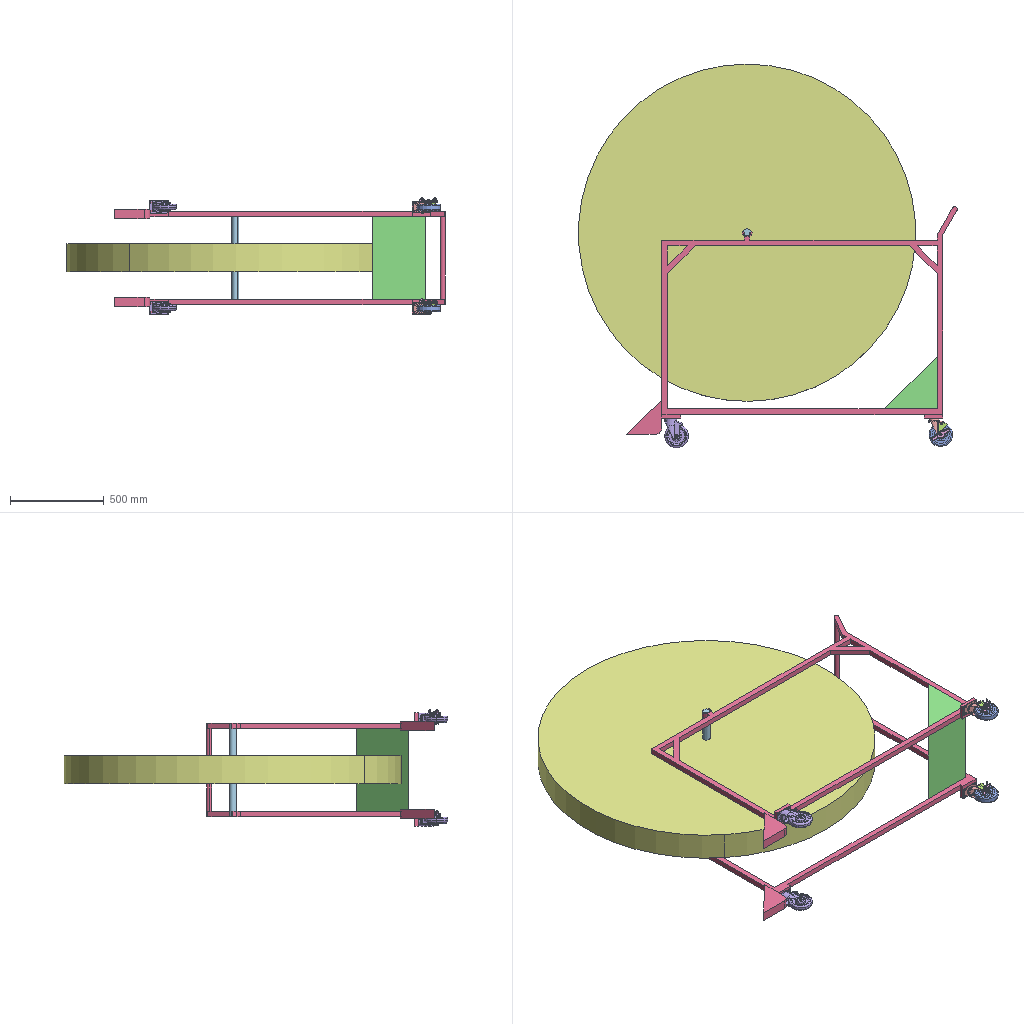Assembly | SolidWorks | 13 different items | 20 placed | box 2020 x 2048 x 623 mm
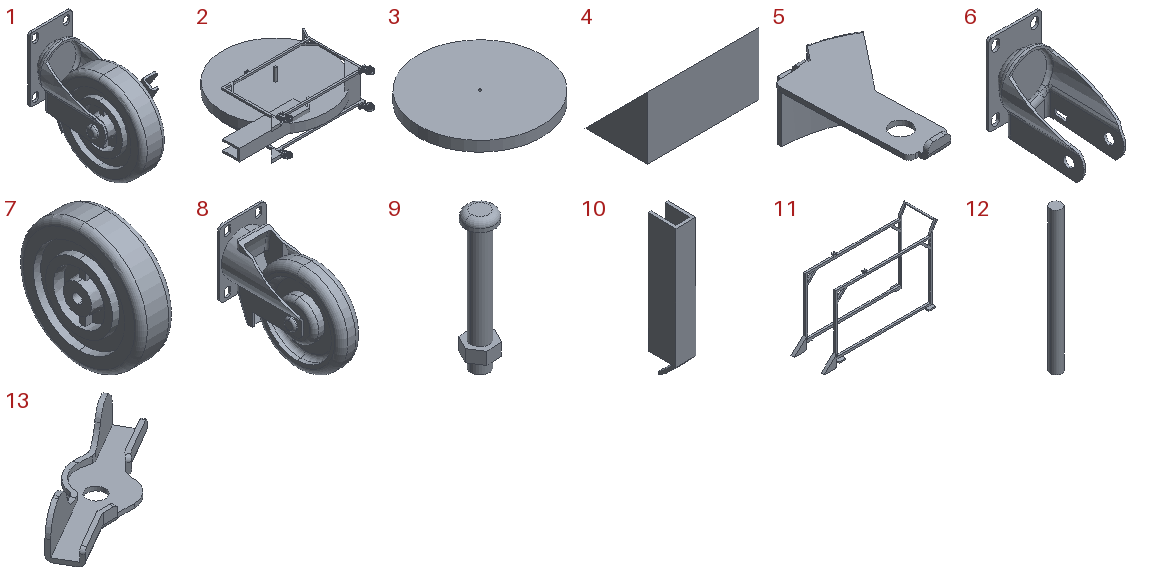Parts list (item | name | quantity | parent item | size | volume | features):
1 | (subassembly) | x2 | - | 82.741 x 151.003 x 143.701 mm | 434028 mm3 | features AEMSimFeature 1, CompositeCurve 1
2 | (subassembly) | x1 | - | 2265 x 1855 x 622.797 mm | 442404059 mm3 | -
3 | - | x1 | - | 1800 x 1800 x 150 mm | 381515012 mm3 | features Extrusion 1, ICE 1
4 | - | x1 | - | 500 x 280 x 280 mm | 19600000 mm3 | features ICE 4, Extrusion 1
5 | - | x2 | in 1 | 48.773 x 87.122 x 45.946 mm | 8989 mm3 | features Fillet 2, ICE 2, SM3dBend 2, FlatPattern 1, SMBaseFlange 1, SheetMetal 1
6 | - | x2 | in 1 | 62.612 x 104.648 x 97.984 mm | 58421 mm3 | features ICE 8, Fillet 5, Extrusion 1, RevCut 1, Revolution 1, Shell 1
7 | - | x2 | in 1 | 37.592 x 125.73 x 125.73 mm | 351247 mm3 | features Cut 2, Draft 2, ICE 2, BossThin 1, Extrusion 1, Fillet 1, MirrorPattern 1
8 | - | x2 | - | 66.675 x 158.75 x 142.081 mm | 379574 mm3 | features ICE 12, Fillet 8, MirrorPattern 5, Extrusion 1, RevCut 1
9 | - | x2 | in 1 | 16.107 x 15.24 x 71.12 mm | 6159 mm3 | features ICE 2, Extrusion 1, Fillet 1
10 | - | x1 | - | 200 x 280 x 1354 mm | 26886001 mm3 | features ICE 3, Extrusion 1
11 | - | x1 | - | 1767 x 605.941 x 1214 mm | 12147544 mm3 | features ICE 12, MirrorPattern 4, Extrusion 1, Fillet 1
12 | - | x1 | - | 40 x 40 x 500 mm | 628319 mm3 | features Extrusion 1
13 | - | x2 | in 1 | 96.878 x 66.198 x 24.765 mm | 9212 mm3 | features Fillet 4, ICE 4, Cut 1, FlatPattern 1, SMBaseFlange 1, SheetMetal 1
Mates (type | each side: item.copy, entity, surface, feature):
In the top assembly
Coincident | 4.1 face plane Boss-Extrude1 | 11.1 face plane Boss-Extrude1 | 2 times
Coincident | 11.1 face plane Boss-Extrude1 | 12.1 face plane Boss-Extrude1
Concentric | 12.1 face cylinder Boss-Extrude1 | 3.1 face cylinder Cut-Extrude1
Coincident | 4.1 face plane Boss-Extrude1 | 11.1 face plane Boss-Extrude2
DistanceDim | 11.1 face plane Boss-Extrude1 | 3.1 face plane Boss-Extrude1
Parallel | 11.1 face plane Boss-Extrude8 | 10.1 face plane Boss-Extrude1
Parallel | 11.1 face plane Boss-Extrude11 | 10.1 face plane Boss-Extrude1
DistanceDim | 11.1 face plane Boss-Extrude11 | 10.1 face plane Boss-Extrude1
Coincident | 8.1 face plane Extrude1 | 11.1 face plane Boss-Extrude12 | 3 times
Coincident | 6.1 face plane Boss-Extrude3 | 11.1 face plane Boss-Extrude12 | 2 times
Coincident | 6.1 face plane Boss-Extrude3 | 11.1 face plane Boss-Extrude1
Coincident | 6.2 face plane Boss-Extrude3 | 11.1 face plane Boss-Extrude12 | 2 times
Coincident | 6.2 face plane Boss-Extrude3 | 11.1 face plane Boss-Extrude1
Coincident | 11.1 face plane Boss-Extrude1 | 10.1 face plane Boss-Extrude1
DistanceDim | 10.1 face plane Boss-Extrude1 | 11.1 face plane Boss-Extrude1
Coincident | 8.2 face plane Extrude1 | 11.1 face plane Boss-Extrude12 | 3 times
Concentric | 11.1 face cylinder Boss-Extrude7 | 12.1 face cylinder Boss-Extrude1
In subassembly 1
InPlace | 6.3 face plane Boss-Extrude2 | 5.1 plane
InPlace | 5.1 face plane Base-Flange1 | 1.1 plane
Concentric | 5.1 edge | 1.1 face
Coincident | 5.1 face plane Base-Flange1 | 1.1 face
InPlace | 5.1 face plane Base-Flange1 | 13.1 plane
InPlace | 6.3 face plane Boss-Extrude2 | 9.1 plane